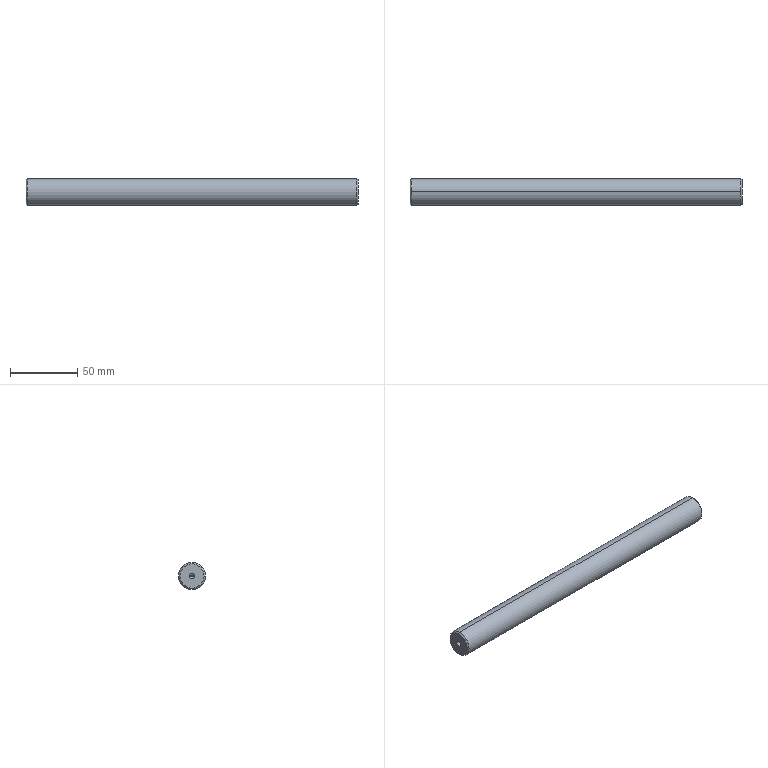Part | STEP file | 06-39 Heat-shrink tube guide shaft | 1 solid | 16 faces | box 246 x 20 x 20 mm | volume 76812 mm3 | cone 8 | cylinder 6 | plane 2 | commonest cylinder face diameters 4.2 x4 20 x2